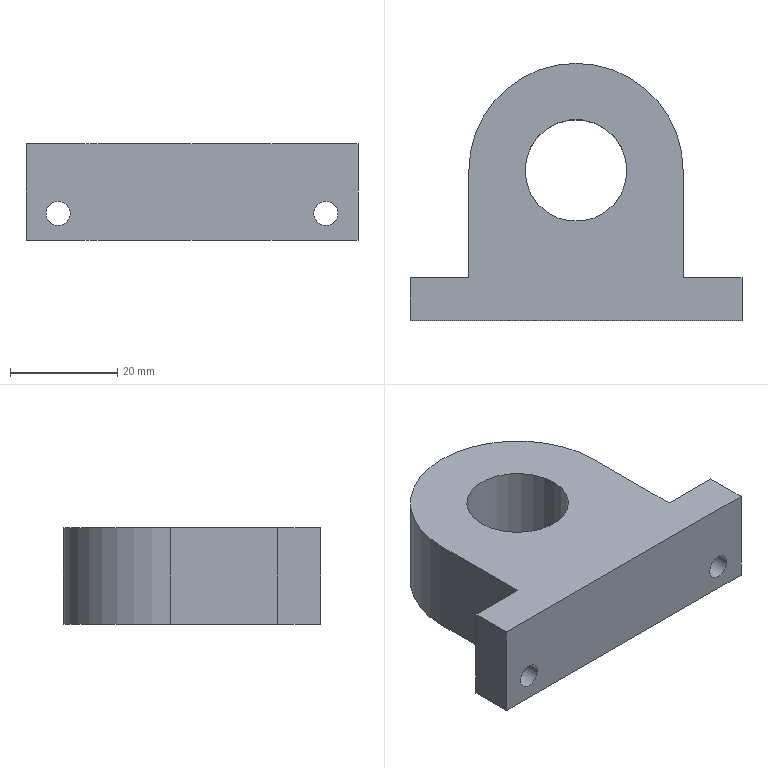Part | Creo | features CURVE 3, DATUM PLANE 3, CUT 2, COORDINATE SYSTEM 1, PROTRUSION 1 | 1 solid | 16 faces | box 62 x 48 x 18 mm | volume 29280 mm3 | plane 9 | cylinder 7 | commonest cylinder face diameters 4.5 x4 19 x2 40 x1
STEP:
#1=CARTESIAN_POINT('',(0.,0.,0.));
#2=DIRECTION('',(0.,0.,1.));
#3=DIRECTION('',(1.,0.,0.));
#4=AXIS2_PLACEMENT_3D('',#1,#2,#3);
#5=CARTESIAN_POINT('',(20.,28.,0.));
#6=VERTEX_POINT('',#5);
#7=CARTESIAN_POINT('',(-20.,28.,0.));
#8=VERTEX_POINT('',#7);
#9=CARTESIAN_POINT('',(0.,28.,0.));
#10=DIRECTION('',(0.,0.,1.));
#11=DIRECTION('',(1.,0.,0.));
#12=AXIS2_PLACEMENT_3D('',#9,#10,#11);
#13=CIRCLE('',#12,20.);
#14=EDGE_CURVE('',#6,#8,#13,.T.);
#15=ORIENTED_EDGE('',*,*,#14,.T.);
#16=CARTESIAN_POINT('',(-20.,8.,0.));
#17=VERTEX_POINT('',#16);
#18=CARTESIAN_POINT('',(-20.,28.,0.));
#19=DIRECTION('',(0.,-1.,0.));
#20=VECTOR('',#19,20.);
#21=LINE('',#18,#20);
#22=EDGE_CURVE('',#8,#17,#21,.T.);
#23=ORIENTED_EDGE('',*,*,#22,.T.);
#24=CARTESIAN_POINT('',(-31.,8.,0.));
#25=VERTEX_POINT('',#24);
#26=CARTESIAN_POINT('',(-20.,8.,0.));
#27=DIRECTION('',(-1.,0.,0.));
#28=VECTOR('',#27,11.);
#29=LINE('',#26,#28);
#30=EDGE_CURVE('',#17,#25,#29,.T.);
#31=ORIENTED_EDGE('',*,*,#30,.T.);
#32=CARTESIAN_POINT('',(-31.,0.,0.));
#33=VERTEX_POINT('',#32);
#34=CARTESIAN_POINT('',(-31.,8.,0.));
#35=DIRECTION('',(0.,-1.,0.));
#36=VECTOR('',#35,8.);
#37=LINE('',#34,#36);
#38=EDGE_CURVE('',#25,#33,#37,.T.);
#39=ORIENTED_EDGE('',*,*,#38,.T.);
#40=CARTESIAN_POINT('',(31.,0.,0.));
#41=VERTEX_POINT('',#40);
#42=CARTESIAN_POINT('',(-31.,0.,0.));
#43=DIRECTION('',(1.,0.,0.));
#44=VECTOR('',#43,62.);
#45=LINE('',#42,#44);
#46=EDGE_CURVE('',#33,#41,#45,.T.);
#47=ORIENTED_EDGE('',*,*,#46,.T.);
#48=CARTESIAN_POINT('',(31.,8.,0.));
#49=VERTEX_POINT('',#48);
#50=CARTESIAN_POINT('',(31.,0.,0.));
#51=DIRECTION('',(0.,1.,0.));
#52=VECTOR('',#51,8.);
#53=LINE('',#50,#52);
#54=EDGE_CURVE('',#41,#49,#53,.T.);
#55=ORIENTED_EDGE('',*,*,#54,.T.);
#56=CARTESIAN_POINT('',(20.,8.,0.));
#57=VERTEX_POINT('',#56);
#58=CARTESIAN_POINT('',(31.,8.,0.));
#59=DIRECTION('',(-1.,0.,0.));
#60=VECTOR('',#59,11.);
#61=LINE('',#58,#60);
#62=EDGE_CURVE('',#49,#57,#61,.T.);
#63=ORIENTED_EDGE('',*,*,#62,.T.);
#64=CARTESIAN_POINT('',(20.,8.,0.));
#65=DIRECTION('',(0.,1.,0.));
#66=VECTOR('',#65,20.);
#67=LINE('',#64,#66);
#68=EDGE_CURVE('',#57,#6,#67,.T.);
#69=ORIENTED_EDGE('',*,*,#68,.T.);
#70=EDGE_LOOP('',(#15,#23,#31,#39,#47,#55,#63,#69));
#71=FACE_OUTER_BOUND('',#70,.F.);
#72=CARTESIAN_POINT('',(-9.5,28.,0.));
#73=VERTEX_POINT('',#72);
#74=CARTESIAN_POINT('',(9.5,28.,0.));
#75=VERTEX_POINT('',#74);
#76=CARTESIAN_POINT('',(0.,28.,0.));
#77=DIRECTION('',(0.,0.,-1.));
#78=DIRECTION('',(-1.,0.,0.));
#79=AXIS2_PLACEMENT_3D('',#76,#77,#78);
#80=CIRCLE('',#79,9.5);
#81=EDGE_CURVE('',#73,#75,#80,.T.);
#82=ORIENTED_EDGE('',*,*,#81,.T.);
#83=CARTESIAN_POINT('',(0.,28.,0.));
#84=DIRECTION('',(0.,0.,-1.));
#85=DIRECTION('',(1.,0.,0.));
#86=AXIS2_PLACEMENT_3D('',#83,#84,#85);
#87=CIRCLE('',#86,9.5);
#88=EDGE_CURVE('',#75,#73,#87,.T.);
#89=ORIENTED_EDGE('',*,*,#88,.T.);
#90=EDGE_LOOP('',(#82,#89));
#91=FACE_BOUND('',#90,.F.);
#92=CARTESIAN_POINT('',(0.,0.,0.));
#93=DIRECTION('',(0.,0.,1.));
#94=DIRECTION('',(1.,0.,0.));
#95=AXIS2_PLACEMENT_3D('',#92,#93,#94);
#96=PLANE('',#95);
#97=ADVANCED_FACE('',(#71,#91),#96,.F.);
#98=ORIENTED_EDGE('',*,*,#14,.F.);
#99=CARTESIAN_POINT('',(20.,28.,18.));
#100=VERTEX_POINT('',#99);
#101=CARTESIAN_POINT('',(20.,28.,0.));
#102=DIRECTION('',(0.,0.,1.));
#103=VECTOR('',#102,18.);
#104=LINE('',#101,#103);
#105=EDGE_CURVE('',#6,#100,#104,.T.);
#106=ORIENTED_EDGE('',*,*,#105,.T.);
#107=CARTESIAN_POINT('',(-20.,28.,18.));
#108=VERTEX_POINT('',#107);
#109=CARTESIAN_POINT('',(0.,28.,18.));
#110=DIRECTION('',(0.,0.,1.));
#111=DIRECTION('',(1.,0.,0.));
#112=AXIS2_PLACEMENT_3D('',#109,#110,#111);
#113=CIRCLE('',#112,20.);
#114=EDGE_CURVE('',#100,#108,#113,.T.);
#115=ORIENTED_EDGE('',*,*,#114,.T.);
#116=CARTESIAN_POINT('',(-20.,28.,0.));
#117=DIRECTION('',(0.,0.,1.));
#118=VECTOR('',#117,18.);
#119=LINE('',#116,#118);
#120=EDGE_CURVE('',#8,#108,#119,.T.);
#121=ORIENTED_EDGE('',*,*,#120,.F.);
#122=EDGE_LOOP('',(#98,#106,#115,#121));
#123=FACE_OUTER_BOUND('',#122,.F.);
#124=CARTESIAN_POINT('',(0.,28.,0.));
#125=DIRECTION('',(0.,0.,1.));
#126=DIRECTION('',(1.,0.,0.));
#127=AXIS2_PLACEMENT_3D('',#124,#125,#126);
#128=CYLINDRICAL_SURFACE('',#127,20.);
#129=ADVANCED_FACE('',(#123),#128,.T.);
#130=ORIENTED_EDGE('',*,*,#68,.F.);
#131=CARTESIAN_POINT('',(20.,8.,18.));
#132=VERTEX_POINT('',#131);
#133=CARTESIAN_POINT('',(20.,8.,0.));
#134=DIRECTION('',(0.,0.,1.));
#135=VECTOR('',#134,18.);
#136=LINE('',#133,#135);
#137=EDGE_CURVE('',#57,#132,#136,.T.);
#138=ORIENTED_EDGE('',*,*,#137,.T.);
#139=CARTESIAN_POINT('',(20.,8.,18.));
#140=DIRECTION('',(0.,1.,0.));
#141=VECTOR('',#140,20.);
#142=LINE('',#139,#141);
#143=EDGE_CURVE('',#132,#100,#142,.T.);
#144=ORIENTED_EDGE('',*,*,#143,.T.);
#145=ORIENTED_EDGE('',*,*,#105,.F.);
#146=EDGE_LOOP('',(#130,#138,#144,#145));
#147=FACE_OUTER_BOUND('',#146,.F.);
#148=CARTESIAN_POINT('',(20.,8.,0.));
#149=DIRECTION('',(1.,0.,0.));
#150=DIRECTION('',(0.,1.,0.));
#151=AXIS2_PLACEMENT_3D('',#148,#149,#150);
#152=PLANE('',#151);
#153=ADVANCED_FACE('',(#147),#152,.T.);
#154=ORIENTED_EDGE('',*,*,#62,.F.);
#155=CARTESIAN_POINT('',(31.,8.,18.));
#156=VERTEX_POINT('',#155);
#157=CARTESIAN_POINT('',(31.,8.,0.));
#158=DIRECTION('',(0.,0.,1.));
#159=VECTOR('',#158,18.);
#160=LINE('',#157,#159);
#161=EDGE_CURVE('',#49,#156,#160,.T.);
#162=ORIENTED_EDGE('',*,*,#161,.T.);
#163=CARTESIAN_POINT('',(31.,8.,18.));
#164=DIRECTION('',(-1.,0.,0.));
#165=VECTOR('',#164,11.);
#166=LINE('',#163,#165);
#167=EDGE_CURVE('',#156,#132,#166,.T.);
#168=ORIENTED_EDGE('',*,*,#167,.T.);
#169=ORIENTED_EDGE('',*,*,#137,.F.);
#170=EDGE_LOOP('',(#154,#162,#168,#169));
#171=FACE_OUTER_BOUND('',#170,.F.);
#172=CARTESIAN_POINT('',(27.25,8.,5.));
#173=VERTEX_POINT('',#172);
#174=CARTESIAN_POINT('',(22.75,8.,5.));
#175=VERTEX_POINT('',#174);
#176=CARTESIAN_POINT('',(25.,8.,5.));
#177=DIRECTION('',(0.,1.,0.));
#178=DIRECTION('',(1.,0.,0.));
#179=AXIS2_PLACEMENT_3D('',#176,#177,#178);
#180=CIRCLE('',#179,2.25);
#181=EDGE_CURVE('',#173,#175,#180,.T.);
#182=ORIENTED_EDGE('',*,*,#181,.T.);
#183=CARTESIAN_POINT('',(25.,8.,5.));
#184=DIRECTION('',(0.,1.,0.));
#185=DIRECTION('',(-1.,0.,0.));
#186=AXIS2_PLACEMENT_3D('',#183,#184,#185);
#187=CIRCLE('',#186,2.25);
#188=EDGE_CURVE('',#175,#173,#187,.T.);
#189=ORIENTED_EDGE('',*,*,#188,.T.);
#190=EDGE_LOOP('',(#182,#189));
#191=FACE_BOUND('',#190,.F.);
#192=CARTESIAN_POINT('',(31.,8.,0.));
#193=DIRECTION('',(0.,1.,0.));
#194=DIRECTION('',(-1.,0.,0.));
#195=AXIS2_PLACEMENT_3D('',#192,#193,#194);
#196=PLANE('',#195);
#197=ADVANCED_FACE('',(#171,#191),#196,.T.);
#198=ORIENTED_EDGE('',*,*,#54,.F.);
#199=CARTESIAN_POINT('',(31.,0.,18.));
#200=VERTEX_POINT('',#199);
#201=CARTESIAN_POINT('',(31.,0.,0.));
#202=DIRECTION('',(0.,0.,1.));
#203=VECTOR('',#202,18.);
#204=LINE('',#201,#203);
#205=EDGE_CURVE('',#41,#200,#204,.T.);
#206=ORIENTED_EDGE('',*,*,#205,.T.);
#207=CARTESIAN_POINT('',(31.,0.,18.));
#208=DIRECTION('',(0.,1.,0.));
#209=VECTOR('',#208,8.);
#210=LINE('',#207,#209);
#211=EDGE_CURVE('',#200,#156,#210,.T.);
#212=ORIENTED_EDGE('',*,*,#211,.T.);
#213=ORIENTED_EDGE('',*,*,#161,.F.);
#214=EDGE_LOOP('',(#198,#206,#212,#213));
#215=FACE_OUTER_BOUND('',#214,.F.);
#216=CARTESIAN_POINT('',(31.,0.,0.));
#217=DIRECTION('',(1.,0.,0.));
#218=DIRECTION('',(0.,1.,0.));
#219=AXIS2_PLACEMENT_3D('',#216,#217,#218);
#220=PLANE('',#219);
#221=ADVANCED_FACE('',(#215),#220,.T.);
#222=ORIENTED_EDGE('',*,*,#46,.F.);
#223=CARTESIAN_POINT('',(-31.,0.,18.));
#224=VERTEX_POINT('',#223);
#225=CARTESIAN_POINT('',(-31.,0.,0.));
#226=DIRECTION('',(0.,0.,1.));
#227=VECTOR('',#226,18.);
#228=LINE('',#225,#227);
#229=EDGE_CURVE('',#33,#224,#228,.T.);
#230=ORIENTED_EDGE('',*,*,#229,.T.);
#231=CARTESIAN_POINT('',(-31.,0.,18.));
#232=DIRECTION('',(1.,0.,0.));
#233=VECTOR('',#232,62.);
#234=LINE('',#231,#233);
#235=EDGE_CURVE('',#224,#200,#234,.T.);
#236=ORIENTED_EDGE('',*,*,#235,.T.);
#237=ORIENTED_EDGE('',*,*,#205,.F.);
#238=EDGE_LOOP('',(#222,#230,#236,#237));
#239=FACE_OUTER_BOUND('',#238,.F.);
#240=CARTESIAN_POINT('',(27.25,0.,5.));
#241=VERTEX_POINT('',#240);
#242=CARTESIAN_POINT('',(22.75,0.,5.));
#243=VERTEX_POINT('',#242);
#244=CARTESIAN_POINT('',(25.,0.,5.));
#245=DIRECTION('',(0.,1.,0.));
#246=DIRECTION('',(1.,0.,0.));
#247=AXIS2_PLACEMENT_3D('',#244,#245,#246);
#248=CIRCLE('',#247,2.25);
#249=EDGE_CURVE('',#241,#243,#248,.T.);
#250=ORIENTED_EDGE('',*,*,#249,.F.);
#251=CARTESIAN_POINT('',(25.,0.,5.));
#252=DIRECTION('',(0.,1.,0.));
#253=DIRECTION('',(-1.,0.,0.));
#254=AXIS2_PLACEMENT_3D('',#251,#252,#253);
#255=CIRCLE('',#254,2.25);
#256=EDGE_CURVE('',#243,#241,#255,.T.);
#257=ORIENTED_EDGE('',*,*,#256,.F.);
#258=EDGE_LOOP('',(#250,#257));
#259=FACE_BOUND('',#258,.F.);
#260=CARTESIAN_POINT('',(-22.75,0.,5.));
#261=VERTEX_POINT('',#260);
#262=CARTESIAN_POINT('',(-27.25,0.,5.));
#263=VERTEX_POINT('',#262);
#264=CARTESIAN_POINT('',(-25.,0.,5.));
#265=DIRECTION('',(0.,1.,0.));
#266=DIRECTION('',(1.,0.,0.));
#267=AXIS2_PLACEMENT_3D('',#264,#265,#266);
#268=CIRCLE('',#267,2.25);
#269=EDGE_CURVE('',#261,#263,#268,.T.);
#270=ORIENTED_EDGE('',*,*,#269,.F.);
#271=CARTESIAN_POINT('',(-25.,0.,5.));
#272=DIRECTION('',(0.,1.,0.));
#273=DIRECTION('',(-1.,0.,0.));
#274=AXIS2_PLACEMENT_3D('',#271,#272,#273);
#275=CIRCLE('',#274,2.25);
#276=EDGE_CURVE('',#263,#261,#275,.T.);
#277=ORIENTED_EDGE('',*,*,#276,.F.);
#278=EDGE_LOOP('',(#270,#277));
#279=FACE_BOUND('',#278,.F.);
#280=CARTESIAN_POINT('',(-31.,0.,0.));
#281=DIRECTION('',(0.,-1.,0.));
#282=DIRECTION('',(1.,0.,0.));
#283=AXIS2_PLACEMENT_3D('',#280,#281,#282);
#284=PLANE('',#283);
#285=ADVANCED_FACE('',(#239,#259,#279),#284,.T.);
#286=ORIENTED_EDGE('',*,*,#38,.F.);
#287=CARTESIAN_POINT('',(-31.,8.,18.));
#288=VERTEX_POINT('',#287);
#289=CARTESIAN_POINT('',(-31.,8.,0.));
#290=DIRECTION('',(0.,0.,1.));
#291=VECTOR('',#290,18.);
#292=LINE('',#289,#291);
#293=EDGE_CURVE('',#25,#288,#292,.T.);
#294=ORIENTED_EDGE('',*,*,#293,.T.);
#295=CARTESIAN_POINT('',(-31.,8.,18.));
#296=DIRECTION('',(0.,-1.,0.));
#297=VECTOR('',#296,8.);
#298=LINE('',#295,#297);
#299=EDGE_CURVE('',#288,#224,#298,.T.);
#300=ORIENTED_EDGE('',*,*,#299,.T.);
#301=ORIENTED_EDGE('',*,*,#229,.F.);
#302=EDGE_LOOP('',(#286,#294,#300,#301));
#303=FACE_OUTER_BOUND('',#302,.F.);
#304=CARTESIAN_POINT('',(-31.,8.,0.));
#305=DIRECTION('',(-1.,0.,0.));
#306=DIRECTION('',(0.,-1.,0.));
#307=AXIS2_PLACEMENT_3D('',#304,#305,#306);
#308=PLANE('',#307);
#309=ADVANCED_FACE('',(#303),#308,.T.);
#310=ORIENTED_EDGE('',*,*,#30,.F.);
#311=CARTESIAN_POINT('',(-20.,8.,18.));
#312=VERTEX_POINT('',#311);
#313=CARTESIAN_POINT('',(-20.,8.,0.));
#314=DIRECTION('',(0.,0.,1.));
#315=VECTOR('',#314,18.);
#316=LINE('',#313,#315);
#317=EDGE_CURVE('',#17,#312,#316,.T.);
#318=ORIENTED_EDGE('',*,*,#317,.T.);
#319=CARTESIAN_POINT('',(-20.,8.,18.));
#320=DIRECTION('',(-1.,0.,0.));
#321=VECTOR('',#320,11.);
#322=LINE('',#319,#321);
#323=EDGE_CURVE('',#312,#288,#322,.T.);
#324=ORIENTED_EDGE('',*,*,#323,.T.);
#325=ORIENTED_EDGE('',*,*,#293,.F.);
#326=EDGE_LOOP('',(#310,#318,#324,#325));
#327=FACE_OUTER_BOUND('',#326,.F.);
#328=CARTESIAN_POINT('',(-22.75,8.,5.));
#329=VERTEX_POINT('',#328);
#330=CARTESIAN_POINT('',(-27.25,8.,5.));
#331=VERTEX_POINT('',#330);
#332=CARTESIAN_POINT('',(-25.,8.,5.));
#333=DIRECTION('',(0.,1.,0.));
#334=DIRECTION('',(1.,0.,0.));
#335=AXIS2_PLACEMENT_3D('',#332,#333,#334);
#336=CIRCLE('',#335,2.25);
#337=EDGE_CURVE('',#329,#331,#336,.T.);
#338=ORIENTED_EDGE('',*,*,#337,.T.);
#339=CARTESIAN_POINT('',(-25.,8.,5.));
#340=DIRECTION('',(0.,1.,0.));
#341=DIRECTION('',(-1.,0.,0.));
#342=AXIS2_PLACEMENT_3D('',#339,#340,#341);
#343=CIRCLE('',#342,2.25);
#344=EDGE_CURVE('',#331,#329,#343,.T.);
#345=ORIENTED_EDGE('',*,*,#344,.T.);
#346=EDGE_LOOP('',(#338,#345));
#347=FACE_BOUND('',#346,.F.);
#348=CARTESIAN_POINT('',(-20.,8.,0.));
#349=DIRECTION('',(0.,1.,0.));
#350=DIRECTION('',(-1.,0.,0.));
#351=AXIS2_PLACEMENT_3D('',#348,#349,#350);
#352=PLANE('',#351);
#353=ADVANCED_FACE('',(#327,#347),#352,.T.);
#354=ORIENTED_EDGE('',*,*,#22,.F.);
#355=ORIENTED_EDGE('',*,*,#120,.T.);
#356=CARTESIAN_POINT('',(-20.,28.,18.));
#357=DIRECTION('',(0.,-1.,0.));
#358=VECTOR('',#357,20.);
#359=LINE('',#356,#358);
#360=EDGE_CURVE('',#108,#312,#359,.T.);
#361=ORIENTED_EDGE('',*,*,#360,.T.);
#362=ORIENTED_EDGE('',*,*,#317,.F.);
#363=EDGE_LOOP('',(#354,#355,#361,#362));
#364=FACE_OUTER_BOUND('',#363,.F.);
#365=CARTESIAN_POINT('',(-20.,28.,0.));
#366=DIRECTION('',(-1.,0.,0.));
#367=DIRECTION('',(0.,-1.,0.));
#368=AXIS2_PLACEMENT_3D('',#365,#366,#367);
#369=PLANE('',#368);
#370=ADVANCED_FACE('',(#364),#369,.T.);
#371=ORIENTED_EDGE('',*,*,#114,.F.);
#372=ORIENTED_EDGE('',*,*,#143,.F.);
#373=ORIENTED_EDGE('',*,*,#167,.F.);
#374=ORIENTED_EDGE('',*,*,#211,.F.);
#375=ORIENTED_EDGE('',*,*,#235,.F.);
#376=ORIENTED_EDGE('',*,*,#299,.F.);
#377=ORIENTED_EDGE('',*,*,#323,.F.);
#378=ORIENTED_EDGE('',*,*,#360,.F.);
#379=EDGE_LOOP('',(#371,#372,#373,#374,#375,#376,#377,#378));
#380=FACE_OUTER_BOUND('',#379,.F.);
#381=CARTESIAN_POINT('',(-9.5,28.,18.));
#382=VERTEX_POINT('',#381);
#383=CARTESIAN_POINT('',(9.5,28.,18.));
#384=VERTEX_POINT('',#383);
#385=CARTESIAN_POINT('',(0.,28.,18.));
#386=DIRECTION('',(0.,0.,-1.));
#387=DIRECTION('',(-1.,0.,0.));
#388=AXIS2_PLACEMENT_3D('',#385,#386,#387);
#389=CIRCLE('',#388,9.5);
#390=EDGE_CURVE('',#382,#384,#389,.T.);
#391=ORIENTED_EDGE('',*,*,#390,.F.);
#392=CARTESIAN_POINT('',(0.,28.,18.));
#393=DIRECTION('',(0.,0.,-1.));
#394=DIRECTION('',(1.,0.,0.));
#395=AXIS2_PLACEMENT_3D('',#392,#393,#394);
#396=CIRCLE('',#395,9.5);
#397=EDGE_CURVE('',#384,#382,#396,.T.);
#398=ORIENTED_EDGE('',*,*,#397,.F.);
#399=EDGE_LOOP('',(#391,#398));
#400=FACE_BOUND('',#399,.F.);
#401=CARTESIAN_POINT('',(0.,0.,18.));
#402=DIRECTION('',(0.,0.,1.));
#403=DIRECTION('',(1.,0.,0.));
#404=AXIS2_PLACEMENT_3D('',#401,#402,#403);
#405=PLANE('',#404);
#406=ADVANCED_FACE('',(#380,#400),#405,.T.);
#407=ORIENTED_EDGE('',*,*,#81,.F.);
#408=CARTESIAN_POINT('',(-9.5,28.,0.));
#409=DIRECTION('',(0.,0.,1.));
#410=VECTOR('',#409,18.);
#411=LINE('',#408,#410);
#412=EDGE_CURVE('',#73,#382,#411,.T.);
#413=ORIENTED_EDGE('',*,*,#412,.T.);
#414=ORIENTED_EDGE('',*,*,#390,.T.);
#415=CARTESIAN_POINT('',(9.5,28.,0.));
#416=DIRECTION('',(0.,0.,1.));
#417=VECTOR('',#416,18.);
#418=LINE('',#415,#417);
#419=EDGE_CURVE('',#75,#384,#418,.T.);
#420=ORIENTED_EDGE('',*,*,#419,.F.);
#421=EDGE_LOOP('',(#407,#413,#414,#420));
#422=FACE_OUTER_BOUND('',#421,.F.);
#423=CARTESIAN_POINT('',(0.,28.,0.));
#424=DIRECTION('',(0.,0.,-1.));
#425=DIRECTION('',(-1.,0.,0.));
#426=AXIS2_PLACEMENT_3D('',#423,#424,#425);
#427=CYLINDRICAL_SURFACE('',#426,9.5);
#428=ADVANCED_FACE('',(#422),#427,.F.);
#429=ORIENTED_EDGE('',*,*,#88,.F.);
#430=ORIENTED_EDGE('',*,*,#419,.T.);
#431=ORIENTED_EDGE('',*,*,#397,.T.);
#432=ORIENTED_EDGE('',*,*,#412,.F.);
#433=EDGE_LOOP('',(#429,#430,#431,#432));
#434=FACE_OUTER_BOUND('',#433,.F.);
#435=CARTESIAN_POINT('',(0.,28.,0.));
#436=DIRECTION('',(0.,0.,-1.));
#437=DIRECTION('',(-1.,0.,0.));
#438=AXIS2_PLACEMENT_3D('',#435,#436,#437);
#439=CYLINDRICAL_SURFACE('',#438,9.5);
#440=ADVANCED_FACE('',(#434),#439,.F.);
#441=ORIENTED_EDGE('',*,*,#337,.F.);
#442=CARTESIAN_POINT('',(-22.75,8.,5.));
#443=DIRECTION('',(0.,-1.,0.));
#444=VECTOR('',#443,8.);
#445=LINE('',#442,#444);
#446=EDGE_CURVE('',#329,#261,#445,.T.);
#447=ORIENTED_EDGE('',*,*,#446,.T.);
#448=ORIENTED_EDGE('',*,*,#269,.T.);
#449=CARTESIAN_POINT('',(-27.25,8.,5.));
#450=DIRECTION('',(0.,-1.,0.));
#451=VECTOR('',#450,8.);
#452=LINE('',#449,#451);
#453=EDGE_CURVE('',#331,#263,#452,.T.);
#454=ORIENTED_EDGE('',*,*,#453,.F.);
#455=EDGE_LOOP('',(#441,#447,#448,#454));
#456=FACE_OUTER_BOUND('',#455,.F.);
#457=CARTESIAN_POINT('',(-25.,8.,5.));
#458=DIRECTION('',(0.,1.,0.));
#459=DIRECTION('',(1.,0.,0.));
#460=AXIS2_PLACEMENT_3D('',#457,#458,#459);
#461=CYLINDRICAL_SURFACE('',#460,2.25);
#462=ADVANCED_FACE('',(#456),#461,.F.);
#463=ORIENTED_EDGE('',*,*,#344,.F.);
#464=ORIENTED_EDGE('',*,*,#453,.T.);
#465=ORIENTED_EDGE('',*,*,#276,.T.);
#466=ORIENTED_EDGE('',*,*,#446,.F.);
#467=EDGE_LOOP('',(#463,#464,#465,#466));
#468=FACE_OUTER_BOUND('',#467,.F.);
#469=CARTESIAN_POINT('',(-25.,8.,5.));
#470=DIRECTION('',(0.,1.,0.));
#471=DIRECTION('',(1.,0.,0.));
#472=AXIS2_PLACEMENT_3D('',#469,#470,#471);
#473=CYLINDRICAL_SURFACE('',#472,2.25);
#474=ADVANCED_FACE('',(#468),#473,.F.);
#475=ORIENTED_EDGE('',*,*,#249,.T.);
#476=CARTESIAN_POINT('',(22.75,8.,5.));
#477=DIRECTION('',(0.,-1.,0.));
#478=VECTOR('',#477,8.);
#479=LINE('',#476,#478);
#480=EDGE_CURVE('',#175,#243,#479,.T.);
#481=ORIENTED_EDGE('',*,*,#480,.F.);
#482=ORIENTED_EDGE('',*,*,#181,.F.);
#483=CARTESIAN_POINT('',(27.25,8.,5.));
#484=DIRECTION('',(0.,-1.,0.));
#485=VECTOR('',#484,8.);
#486=LINE('',#483,#485);
#487=EDGE_CURVE('',#173,#241,#486,.T.);
#488=ORIENTED_EDGE('',*,*,#487,.T.);
#489=EDGE_LOOP('',(#475,#481,#482,#488));
#490=FACE_OUTER_BOUND('',#489,.F.);
#491=CARTESIAN_POINT('',(25.,8.,5.));
#492=DIRECTION('',(0.,1.,0.));
#493=DIRECTION('',(1.,0.,0.));
#494=AXIS2_PLACEMENT_3D('',#491,#492,#493);
#495=CYLINDRICAL_SURFACE('',#494,2.25);
#496=ADVANCED_FACE('',(#490),#495,.F.);
#497=ORIENTED_EDGE('',*,*,#256,.T.);
#498=ORIENTED_EDGE('',*,*,#487,.F.);
#499=ORIENTED_EDGE('',*,*,#188,.F.);
#500=ORIENTED_EDGE('',*,*,#480,.T.);
#501=EDGE_LOOP('',(#497,#498,#499,#500));
#502=FACE_OUTER_BOUND('',#501,.F.);
#503=CARTESIAN_POINT('',(25.,8.,5.));
#504=DIRECTION('',(0.,1.,0.));
#505=DIRECTION('',(1.,0.,0.));
#506=AXIS2_PLACEMENT_3D('',#503,#504,#505);
#507=CYLINDRICAL_SURFACE('',#506,2.25);
#508=ADVANCED_FACE('',(#502),#507,.F.);
#509=CLOSED_SHELL('',(#97,#129,#153,#197,#221,#285,#309,#353,#370,#406,#428,#440,#462,#474,#496,#508));
#510=MANIFOLD_SOLID_BREP('',#509);
#511=(LENGTH_UNIT()NAMED_UNIT(*)SI_UNIT(.MILLI.,.METRE.));
#512=UNCERTAINTY_MEASURE_WITH_UNIT(LENGTH_MEASURE(0.008045),#511,'','');
#513=(NAMED_UNIT(*)PLANE_ANGLE_UNIT()SI_UNIT($,.RADIAN.));
#514=PLANE_ANGLE_MEASURE_WITH_UNIT(PLANE_ANGLE_MEASURE(0.01745),#513);
#515=(CONVERSION_BASED_UNIT('DEGREE',#514)NAMED_UNIT(*)PLANE_ANGLE_UNIT());
#516=(NAMED_UNIT(*)SI_UNIT($,.STERADIAN.)SOLID_ANGLE_UNIT());
#517=(GEOMETRIC_REPRESENTATION_CONTEXT(3)GLOBAL_UNCERTAINTY_ASSIGNED_CONTEXT((#512))GLOBAL_UNIT_ASSIGNED_CONTEXT((#511,#515,#516))REPRESENTATION_CONTEXT('',''));
#518=ADVANCED_BREP_SHAPE_REPRESENTATION('',(#4,#510),#517);